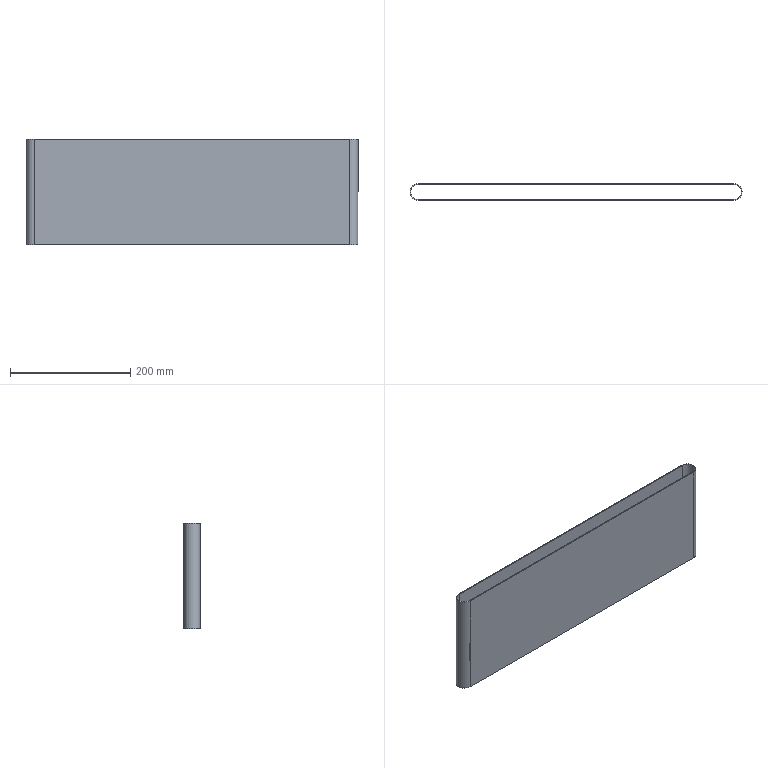Part | SolidWorks | features SplitBody 1 | 1 solid | 12 faces | box 552.3 x 27.3 x 175 mm | volume 208091 mm3 | cylinder 6 | plane 6 | commonest cylinder face diameters 25.2 x3 27.3 x3
STEP:
#1=CARTESIAN_POINT('',(453.475,255.459,-448.416));
#2=VERTEX_POINT('',#1);
#3=CARTESIAN_POINT('',(466.075,242.859,-448.416));
#4=VERTEX_POINT('',#3);
#5=CARTESIAN_POINT('',(453.475,242.859,-448.416));
#6=DIRECTION('',(0.,0.,-1.));
#7=DIRECTION('',(-1.,0.,0.));
#8=AXIS2_PLACEMENT_3D('',#5,#6,#7);
#9=CIRCLE('',#8,12.6);
#10=EDGE_CURVE('',#2,#4,#9,.T.);
#11=ORIENTED_EDGE('',*,*,#10,.T.);
#12=CARTESIAN_POINT('',(466.075,242.859,-273.416));
#13=VERTEX_POINT('',#12);
#14=CARTESIAN_POINT('',(466.075,242.859,-448.416));
#15=DIRECTION('',(0.,0.,1.));
#16=VECTOR('',#15,1000.);
#17=LINE('',#14,#16);
#18=EDGE_CURVE('',#4,#13,#17,.T.);
#19=ORIENTED_EDGE('',*,*,#18,.T.);
#20=CARTESIAN_POINT('',(453.475,255.459,-273.416));
#21=VERTEX_POINT('',#20);
#22=CARTESIAN_POINT('',(453.475,242.859,-273.416));
#23=DIRECTION('',(0.,0.,-1.));
#24=DIRECTION('',(-1.,0.,0.));
#25=AXIS2_PLACEMENT_3D('',#22,#23,#24);
#26=CIRCLE('',#25,12.6);
#27=EDGE_CURVE('',#21,#13,#26,.T.);
#28=ORIENTED_EDGE('',*,*,#27,.F.);
#29=CARTESIAN_POINT('',(453.475,255.459,-448.416));
#30=DIRECTION('',(0.,0.,1.));
#31=VECTOR('',#30,1000.);
#32=LINE('',#29,#31);
#33=EDGE_CURVE('',#2,#21,#32,.T.);
#34=ORIENTED_EDGE('',*,*,#33,.F.);
#35=EDGE_LOOP('',(#11,#19,#28,#34));
#36=FACE_OUTER_BOUND('',#35,.T.);
#37=CARTESIAN_POINT('',(453.475,242.859,-448.416));
#38=DIRECTION('',(0.,0.,1.));
#39=DIRECTION('',(1.,0.,0.));
#40=AXIS2_PLACEMENT_3D('',#37,#38,#39);
#41=CYLINDRICAL_SURFACE('',#40,12.6);
#42=ADVANCED_FACE('',(#36),#41,.F.);
#43=CARTESIAN_POINT('',(467.125,242.859,-448.416));
#44=VERTEX_POINT('',#43);
#45=CARTESIAN_POINT('',(453.475,229.209,-448.416));
#46=VERTEX_POINT('',#45);
#47=CARTESIAN_POINT('',(453.475,242.859,-448.416));
#48=DIRECTION('',(0.,0.,-1.));
#49=DIRECTION('',(-1.,0.,0.));
#50=AXIS2_PLACEMENT_3D('',#47,#48,#49);
#51=CIRCLE('',#50,13.65);
#52=EDGE_CURVE('',#44,#46,#51,.T.);
#53=ORIENTED_EDGE('',*,*,#52,.F.);
#54=CARTESIAN_POINT('',(467.125,242.859,-273.416));
#55=VERTEX_POINT('',#54);
#56=CARTESIAN_POINT('',(467.125,242.859,-448.416));
#57=DIRECTION('',(0.,0.,1.));
#58=VECTOR('',#57,1000.);
#59=LINE('',#56,#58);
#60=EDGE_CURVE('',#44,#55,#59,.T.);
#61=ORIENTED_EDGE('',*,*,#60,.T.);
#62=CARTESIAN_POINT('',(453.475,229.209,-273.416));
#63=VERTEX_POINT('',#62);
#64=CARTESIAN_POINT('',(453.475,242.859,-273.416));
#65=DIRECTION('',(0.,0.,-1.));
#66=DIRECTION('',(-1.,0.,0.));
#67=AXIS2_PLACEMENT_3D('',#64,#65,#66);
#68=CIRCLE('',#67,13.65);
#69=EDGE_CURVE('',#55,#63,#68,.T.);
#70=ORIENTED_EDGE('',*,*,#69,.T.);
#71=CARTESIAN_POINT('',(453.475,229.209,-448.416));
#72=DIRECTION('',(0.,0.,1.));
#73=VECTOR('',#72,1000.);
#74=LINE('',#71,#73);
#75=EDGE_CURVE('',#46,#63,#74,.T.);
#76=ORIENTED_EDGE('',*,*,#75,.F.);
#77=EDGE_LOOP('',(#53,#61,#70,#76));
#78=FACE_OUTER_BOUND('',#77,.T.);
#79=CARTESIAN_POINT('',(453.475,242.859,-448.416));
#80=DIRECTION('',(0.,0.,1.));
#81=DIRECTION('',(1.,0.,0.));
#82=AXIS2_PLACEMENT_3D('',#79,#80,#81);
#83=CYLINDRICAL_SURFACE('',#82,13.65);
#84=ADVANCED_FACE('',(#78),#83,.T.);
#85=CARTESIAN_POINT('',(453.475,256.509,-448.416));
#86=VERTEX_POINT('',#85);
#87=CARTESIAN_POINT('',(453.475,242.859,-448.416));
#88=DIRECTION('',(0.,0.,-1.));
#89=DIRECTION('',(-1.,0.,0.));
#90=AXIS2_PLACEMENT_3D('',#87,#88,#89);
#91=CIRCLE('',#90,13.65);
#92=EDGE_CURVE('',#86,#44,#91,.T.);
#93=ORIENTED_EDGE('',*,*,#92,.T.);
#94=ORIENTED_EDGE('',*,*,#52,.T.);
#95=CARTESIAN_POINT('',(-71.525,229.209,-448.416));
#96=VERTEX_POINT('',#95);
#97=CARTESIAN_POINT('',(453.475,229.209,-448.416));
#98=DIRECTION('',(-1.,0.,0.));
#99=VECTOR('',#98,1000.);
#100=LINE('',#97,#99);
#101=EDGE_CURVE('',#46,#96,#100,.T.);
#102=ORIENTED_EDGE('',*,*,#101,.T.);
#103=CARTESIAN_POINT('',(-71.525,256.509,-448.416));
#104=VERTEX_POINT('',#103);
#105=CARTESIAN_POINT('',(-71.525,242.859,-448.416));
#106=DIRECTION('',(0.,0.,-1.));
#107=DIRECTION('',(-1.,0.,0.));
#108=AXIS2_PLACEMENT_3D('',#105,#106,#107);
#109=CIRCLE('',#108,13.65);
#110=EDGE_CURVE('',#96,#104,#109,.T.);
#111=ORIENTED_EDGE('',*,*,#110,.T.);
#112=CARTESIAN_POINT('',(453.475,256.509,-448.416));
#113=DIRECTION('',(1.,0.,0.));
#114=VECTOR('',#113,1000.);
#115=LINE('',#112,#114);
#116=EDGE_CURVE('',#104,#86,#115,.T.);
#117=ORIENTED_EDGE('',*,*,#116,.T.);
#118=EDGE_LOOP('',(#93,#94,#102,#111,#117));
#119=FACE_OUTER_BOUND('',#118,.T.);
#120=CARTESIAN_POINT('',(453.475,230.259,-448.416));
#121=VERTEX_POINT('',#120);
#122=CARTESIAN_POINT('',(-71.525,230.259,-448.416));
#123=VERTEX_POINT('',#122);
#124=CARTESIAN_POINT('',(453.475,230.259,-448.416));
#125=DIRECTION('',(-1.,0.,0.));
#126=VECTOR('',#125,1000.);
#127=LINE('',#124,#126);
#128=EDGE_CURVE('',#121,#123,#127,.T.);
#129=ORIENTED_EDGE('',*,*,#128,.F.);
#130=CARTESIAN_POINT('',(453.475,242.859,-448.416));
#131=DIRECTION('',(0.,0.,-1.));
#132=DIRECTION('',(-1.,0.,0.));
#133=AXIS2_PLACEMENT_3D('',#130,#131,#132);
#134=CIRCLE('',#133,12.6);
#135=EDGE_CURVE('',#4,#121,#134,.T.);
#136=ORIENTED_EDGE('',*,*,#135,.F.);
#137=ORIENTED_EDGE('',*,*,#10,.F.);
#138=CARTESIAN_POINT('',(-71.525,255.459,-448.416));
#139=VERTEX_POINT('',#138);
#140=CARTESIAN_POINT('',(453.475,255.459,-448.416));
#141=DIRECTION('',(1.,0.,0.));
#142=VECTOR('',#141,1000.);
#143=LINE('',#140,#142);
#144=EDGE_CURVE('',#139,#2,#143,.T.);
#145=ORIENTED_EDGE('',*,*,#144,.F.);
#146=CARTESIAN_POINT('',(-71.525,242.859,-448.416));
#147=DIRECTION('',(0.,0.,-1.));
#148=DIRECTION('',(-1.,0.,0.));
#149=AXIS2_PLACEMENT_3D('',#146,#147,#148);
#150=CIRCLE('',#149,12.6);
#151=EDGE_CURVE('',#123,#139,#150,.T.);
#152=ORIENTED_EDGE('',*,*,#151,.F.);
#153=EDGE_LOOP('',(#129,#136,#137,#145,#152));
#154=FACE_BOUND('',#153,.T.);
#155=CARTESIAN_POINT('',(453.475,242.859,-448.416));
#156=DIRECTION('',(0.,0.,-1.));
#157=DIRECTION('',(-1.,0.,0.));
#158=AXIS2_PLACEMENT_3D('',#155,#156,#157);
#159=PLANE('',#158);
#160=ADVANCED_FACE('',(#119,#154),#159,.T.);
#161=CARTESIAN_POINT('',(453.475,256.509,-273.416));
#162=VERTEX_POINT('',#161);
#163=CARTESIAN_POINT('',(453.475,242.859,-273.416));
#164=DIRECTION('',(0.,0.,-1.));
#165=DIRECTION('',(-1.,0.,0.));
#166=AXIS2_PLACEMENT_3D('',#163,#164,#165);
#167=CIRCLE('',#166,13.65);
#168=EDGE_CURVE('',#162,#55,#167,.T.);
#169=ORIENTED_EDGE('',*,*,#168,.F.);
#170=CARTESIAN_POINT('',(-71.525,256.509,-273.416));
#171=VERTEX_POINT('',#170);
#172=CARTESIAN_POINT('',(453.475,256.509,-273.416));
#173=DIRECTION('',(1.,0.,0.));
#174=VECTOR('',#173,1000.);
#175=LINE('',#172,#174);
#176=EDGE_CURVE('',#171,#162,#175,.T.);
#177=ORIENTED_EDGE('',*,*,#176,.F.);
#178=CARTESIAN_POINT('',(-71.525,229.209,-273.416));
#179=VERTEX_POINT('',#178);
#180=CARTESIAN_POINT('',(-71.525,242.859,-273.416));
#181=DIRECTION('',(0.,0.,-1.));
#182=DIRECTION('',(-1.,0.,0.));
#183=AXIS2_PLACEMENT_3D('',#180,#181,#182);
#184=CIRCLE('',#183,13.65);
#185=EDGE_CURVE('',#179,#171,#184,.T.);
#186=ORIENTED_EDGE('',*,*,#185,.F.);
#187=CARTESIAN_POINT('',(453.475,229.209,-273.416));
#188=DIRECTION('',(-1.,0.,0.));
#189=VECTOR('',#188,1000.);
#190=LINE('',#187,#189);
#191=EDGE_CURVE('',#63,#179,#190,.T.);
#192=ORIENTED_EDGE('',*,*,#191,.F.);
#193=ORIENTED_EDGE('',*,*,#69,.F.);
#194=EDGE_LOOP('',(#169,#177,#186,#192,#193));
#195=FACE_OUTER_BOUND('',#194,.T.);
#196=ORIENTED_EDGE('',*,*,#27,.T.);
#197=CARTESIAN_POINT('',(453.475,230.259,-273.416));
#198=VERTEX_POINT('',#197);
#199=CARTESIAN_POINT('',(453.475,242.859,-273.416));
#200=DIRECTION('',(0.,0.,-1.));
#201=DIRECTION('',(-1.,0.,0.));
#202=AXIS2_PLACEMENT_3D('',#199,#200,#201);
#203=CIRCLE('',#202,12.6);
#204=EDGE_CURVE('',#13,#198,#203,.T.);
#205=ORIENTED_EDGE('',*,*,#204,.T.);
#206=CARTESIAN_POINT('',(-71.525,230.259,-273.416));
#207=VERTEX_POINT('',#206);
#208=CARTESIAN_POINT('',(453.475,230.259,-273.416));
#209=DIRECTION('',(-1.,0.,0.));
#210=VECTOR('',#209,1000.);
#211=LINE('',#208,#210);
#212=EDGE_CURVE('',#198,#207,#211,.T.);
#213=ORIENTED_EDGE('',*,*,#212,.T.);
#214=CARTESIAN_POINT('',(-71.525,255.459,-273.416));
#215=VERTEX_POINT('',#214);
#216=CARTESIAN_POINT('',(-71.525,242.859,-273.416));
#217=DIRECTION('',(0.,0.,-1.));
#218=DIRECTION('',(-1.,0.,0.));
#219=AXIS2_PLACEMENT_3D('',#216,#217,#218);
#220=CIRCLE('',#219,12.6);
#221=EDGE_CURVE('',#207,#215,#220,.T.);
#222=ORIENTED_EDGE('',*,*,#221,.T.);
#223=CARTESIAN_POINT('',(453.475,255.459,-273.416));
#224=DIRECTION('',(1.,0.,0.));
#225=VECTOR('',#224,1000.);
#226=LINE('',#223,#225);
#227=EDGE_CURVE('',#215,#21,#226,.T.);
#228=ORIENTED_EDGE('',*,*,#227,.T.);
#229=EDGE_LOOP('',(#196,#205,#213,#222,#228));
#230=FACE_BOUND('',#229,.T.);
#231=CARTESIAN_POINT('',(453.475,242.859,-273.416));
#232=DIRECTION('',(0.,0.,-1.));
#233=DIRECTION('',(-1.,0.,0.));
#234=AXIS2_PLACEMENT_3D('',#231,#232,#233);
#235=PLANE('',#234);
#236=ADVANCED_FACE('',(#195,#230),#235,.F.);
#237=ORIENTED_EDGE('',*,*,#60,.F.);
#238=ORIENTED_EDGE('',*,*,#92,.F.);
#239=CARTESIAN_POINT('',(453.475,256.509,-448.416));
#240=DIRECTION('',(0.,0.,1.));
#241=VECTOR('',#240,1000.);
#242=LINE('',#239,#241);
#243=EDGE_CURVE('',#86,#162,#242,.T.);
#244=ORIENTED_EDGE('',*,*,#243,.T.);
#245=ORIENTED_EDGE('',*,*,#168,.T.);
#246=EDGE_LOOP('',(#237,#238,#244,#245));
#247=FACE_OUTER_BOUND('',#246,.T.);
#248=CARTESIAN_POINT('',(453.475,242.859,-448.416));
#249=DIRECTION('',(0.,0.,1.));
#250=DIRECTION('',(1.,0.,0.));
#251=AXIS2_PLACEMENT_3D('',#248,#249,#250);
#252=CYLINDRICAL_SURFACE('',#251,13.65);
#253=ADVANCED_FACE('',(#247),#252,.T.);
#254=ORIENTED_EDGE('',*,*,#191,.T.);
#255=CARTESIAN_POINT('',(-71.525,229.209,-448.416));
#256=DIRECTION('',(0.,0.,1.));
#257=VECTOR('',#256,1000.);
#258=LINE('',#255,#257);
#259=EDGE_CURVE('',#96,#179,#258,.T.);
#260=ORIENTED_EDGE('',*,*,#259,.F.);
#261=ORIENTED_EDGE('',*,*,#101,.F.);
#262=ORIENTED_EDGE('',*,*,#75,.T.);
#263=EDGE_LOOP('',(#254,#260,#261,#262));
#264=FACE_OUTER_BOUND('',#263,.T.);
#265=CARTESIAN_POINT('',(453.475,229.209,-448.416));
#266=DIRECTION('',(0.,1.,0.));
#267=DIRECTION('',(0.,0.,-1.));
#268=AXIS2_PLACEMENT_3D('',#265,#266,#267);
#269=PLANE('',#268);
#270=ADVANCED_FACE('',(#264),#269,.F.);
#271=ORIENTED_EDGE('',*,*,#185,.T.);
#272=CARTESIAN_POINT('',(-71.525,256.509,-448.416));
#273=DIRECTION('',(0.,0.,1.));
#274=VECTOR('',#273,1000.);
#275=LINE('',#272,#274);
#276=EDGE_CURVE('',#104,#171,#275,.T.);
#277=ORIENTED_EDGE('',*,*,#276,.F.);
#278=ORIENTED_EDGE('',*,*,#110,.F.);
#279=ORIENTED_EDGE('',*,*,#259,.T.);
#280=EDGE_LOOP('',(#271,#277,#278,#279));
#281=FACE_OUTER_BOUND('',#280,.T.);
#282=CARTESIAN_POINT('',(-71.525,242.859,-448.416));
#283=DIRECTION('',(0.,0.,1.));
#284=DIRECTION('',(1.,0.,0.));
#285=AXIS2_PLACEMENT_3D('',#282,#283,#284);
#286=CYLINDRICAL_SURFACE('',#285,13.65);
#287=ADVANCED_FACE('',(#281),#286,.T.);
#288=ORIENTED_EDGE('',*,*,#176,.T.);
#289=ORIENTED_EDGE('',*,*,#243,.F.);
#290=ORIENTED_EDGE('',*,*,#116,.F.);
#291=ORIENTED_EDGE('',*,*,#276,.T.);
#292=EDGE_LOOP('',(#288,#289,#290,#291));
#293=FACE_OUTER_BOUND('',#292,.T.);
#294=CARTESIAN_POINT('',(453.475,256.509,-448.416));
#295=DIRECTION('',(0.,-1.,0.));
#296=DIRECTION('',(0.,0.,1.));
#297=AXIS2_PLACEMENT_3D('',#294,#295,#296);
#298=PLANE('',#297);
#299=ADVANCED_FACE('',(#293),#298,.F.);
#300=ORIENTED_EDGE('',*,*,#18,.F.);
#301=ORIENTED_EDGE('',*,*,#135,.T.);
#302=CARTESIAN_POINT('',(453.475,230.259,-448.416));
#303=DIRECTION('',(0.,0.,1.));
#304=VECTOR('',#303,1000.);
#305=LINE('',#302,#304);
#306=EDGE_CURVE('',#121,#198,#305,.T.);
#307=ORIENTED_EDGE('',*,*,#306,.T.);
#308=ORIENTED_EDGE('',*,*,#204,.F.);
#309=EDGE_LOOP('',(#300,#301,#307,#308));
#310=FACE_OUTER_BOUND('',#309,.T.);
#311=CARTESIAN_POINT('',(453.475,242.859,-448.416));
#312=DIRECTION('',(0.,0.,1.));
#313=DIRECTION('',(1.,0.,0.));
#314=AXIS2_PLACEMENT_3D('',#311,#312,#313);
#315=CYLINDRICAL_SURFACE('',#314,12.6);
#316=ADVANCED_FACE('',(#310),#315,.F.);
#317=ORIENTED_EDGE('',*,*,#212,.F.);
#318=ORIENTED_EDGE('',*,*,#306,.F.);
#319=ORIENTED_EDGE('',*,*,#128,.T.);
#320=CARTESIAN_POINT('',(-71.525,230.259,-448.416));
#321=DIRECTION('',(0.,0.,1.));
#322=VECTOR('',#321,1000.);
#323=LINE('',#320,#322);
#324=EDGE_CURVE('',#123,#207,#323,.T.);
#325=ORIENTED_EDGE('',*,*,#324,.T.);
#326=EDGE_LOOP('',(#317,#318,#319,#325));
#327=FACE_OUTER_BOUND('',#326,.T.);
#328=CARTESIAN_POINT('',(453.475,230.259,-448.416));
#329=DIRECTION('',(0.,1.,0.));
#330=DIRECTION('',(0.,0.,-1.));
#331=AXIS2_PLACEMENT_3D('',#328,#329,#330);
#332=PLANE('',#331);
#333=ADVANCED_FACE('',(#327),#332,.T.);
#334=ORIENTED_EDGE('',*,*,#221,.F.);
#335=ORIENTED_EDGE('',*,*,#324,.F.);
#336=ORIENTED_EDGE('',*,*,#151,.T.);
#337=CARTESIAN_POINT('',(-71.525,255.459,-448.416));
#338=DIRECTION('',(0.,0.,1.));
#339=VECTOR('',#338,1000.);
#340=LINE('',#337,#339);
#341=EDGE_CURVE('',#139,#215,#340,.T.);
#342=ORIENTED_EDGE('',*,*,#341,.T.);
#343=EDGE_LOOP('',(#334,#335,#336,#342));
#344=FACE_OUTER_BOUND('',#343,.T.);
#345=CARTESIAN_POINT('',(-71.525,242.859,-448.416));
#346=DIRECTION('',(0.,0.,1.));
#347=DIRECTION('',(1.,0.,0.));
#348=AXIS2_PLACEMENT_3D('',#345,#346,#347);
#349=CYLINDRICAL_SURFACE('',#348,12.6);
#350=ADVANCED_FACE('',(#344),#349,.F.);
#351=ORIENTED_EDGE('',*,*,#227,.F.);
#352=ORIENTED_EDGE('',*,*,#341,.F.);
#353=ORIENTED_EDGE('',*,*,#144,.T.);
#354=ORIENTED_EDGE('',*,*,#33,.T.);
#355=EDGE_LOOP('',(#351,#352,#353,#354));
#356=FACE_OUTER_BOUND('',#355,.T.);
#357=CARTESIAN_POINT('',(453.475,255.459,-448.416));
#358=DIRECTION('',(0.,-1.,0.));
#359=DIRECTION('',(0.,0.,1.));
#360=AXIS2_PLACEMENT_3D('',#357,#358,#359);
#361=PLANE('',#360);
#362=ADVANCED_FACE('',(#356),#361,.T.);
#363=CLOSED_SHELL('',(#42,#84,#160,#236,#253,#270,#287,#299,#316,#333,#350,#362));
#364=MANIFOLD_SOLID_BREP('',#363);
#365=CARTESIAN_POINT('',(0.,0.,0.));
#366=DIRECTION('',(0.,0.,1.));
#367=DIRECTION('',(1.,0.,0.));
#368=AXIS2_PLACEMENT_3D('',#365,#366,#367);
#369=(LENGTH_UNIT()NAMED_UNIT(*)SI_UNIT(.MILLI.,.METRE.));
#370=UNCERTAINTY_MEASURE_WITH_UNIT(LENGTH_MEASURE(0.00001),#369,'','');
#371=(NAMED_UNIT(*)PLANE_ANGLE_UNIT()SI_UNIT($,.RADIAN.));
#372=(NAMED_UNIT(*)SI_UNIT($,.STERADIAN.)SOLID_ANGLE_UNIT());
#373=(GEOMETRIC_REPRESENTATION_CONTEXT(3)GLOBAL_UNCERTAINTY_ASSIGNED_CONTEXT((#370))GLOBAL_UNIT_ASSIGNED_CONTEXT((#369,#371,#372))REPRESENTATION_CONTEXT('',''));
#374=ADVANCED_BREP_SHAPE_REPRESENTATION('',(#364,#368),#373);